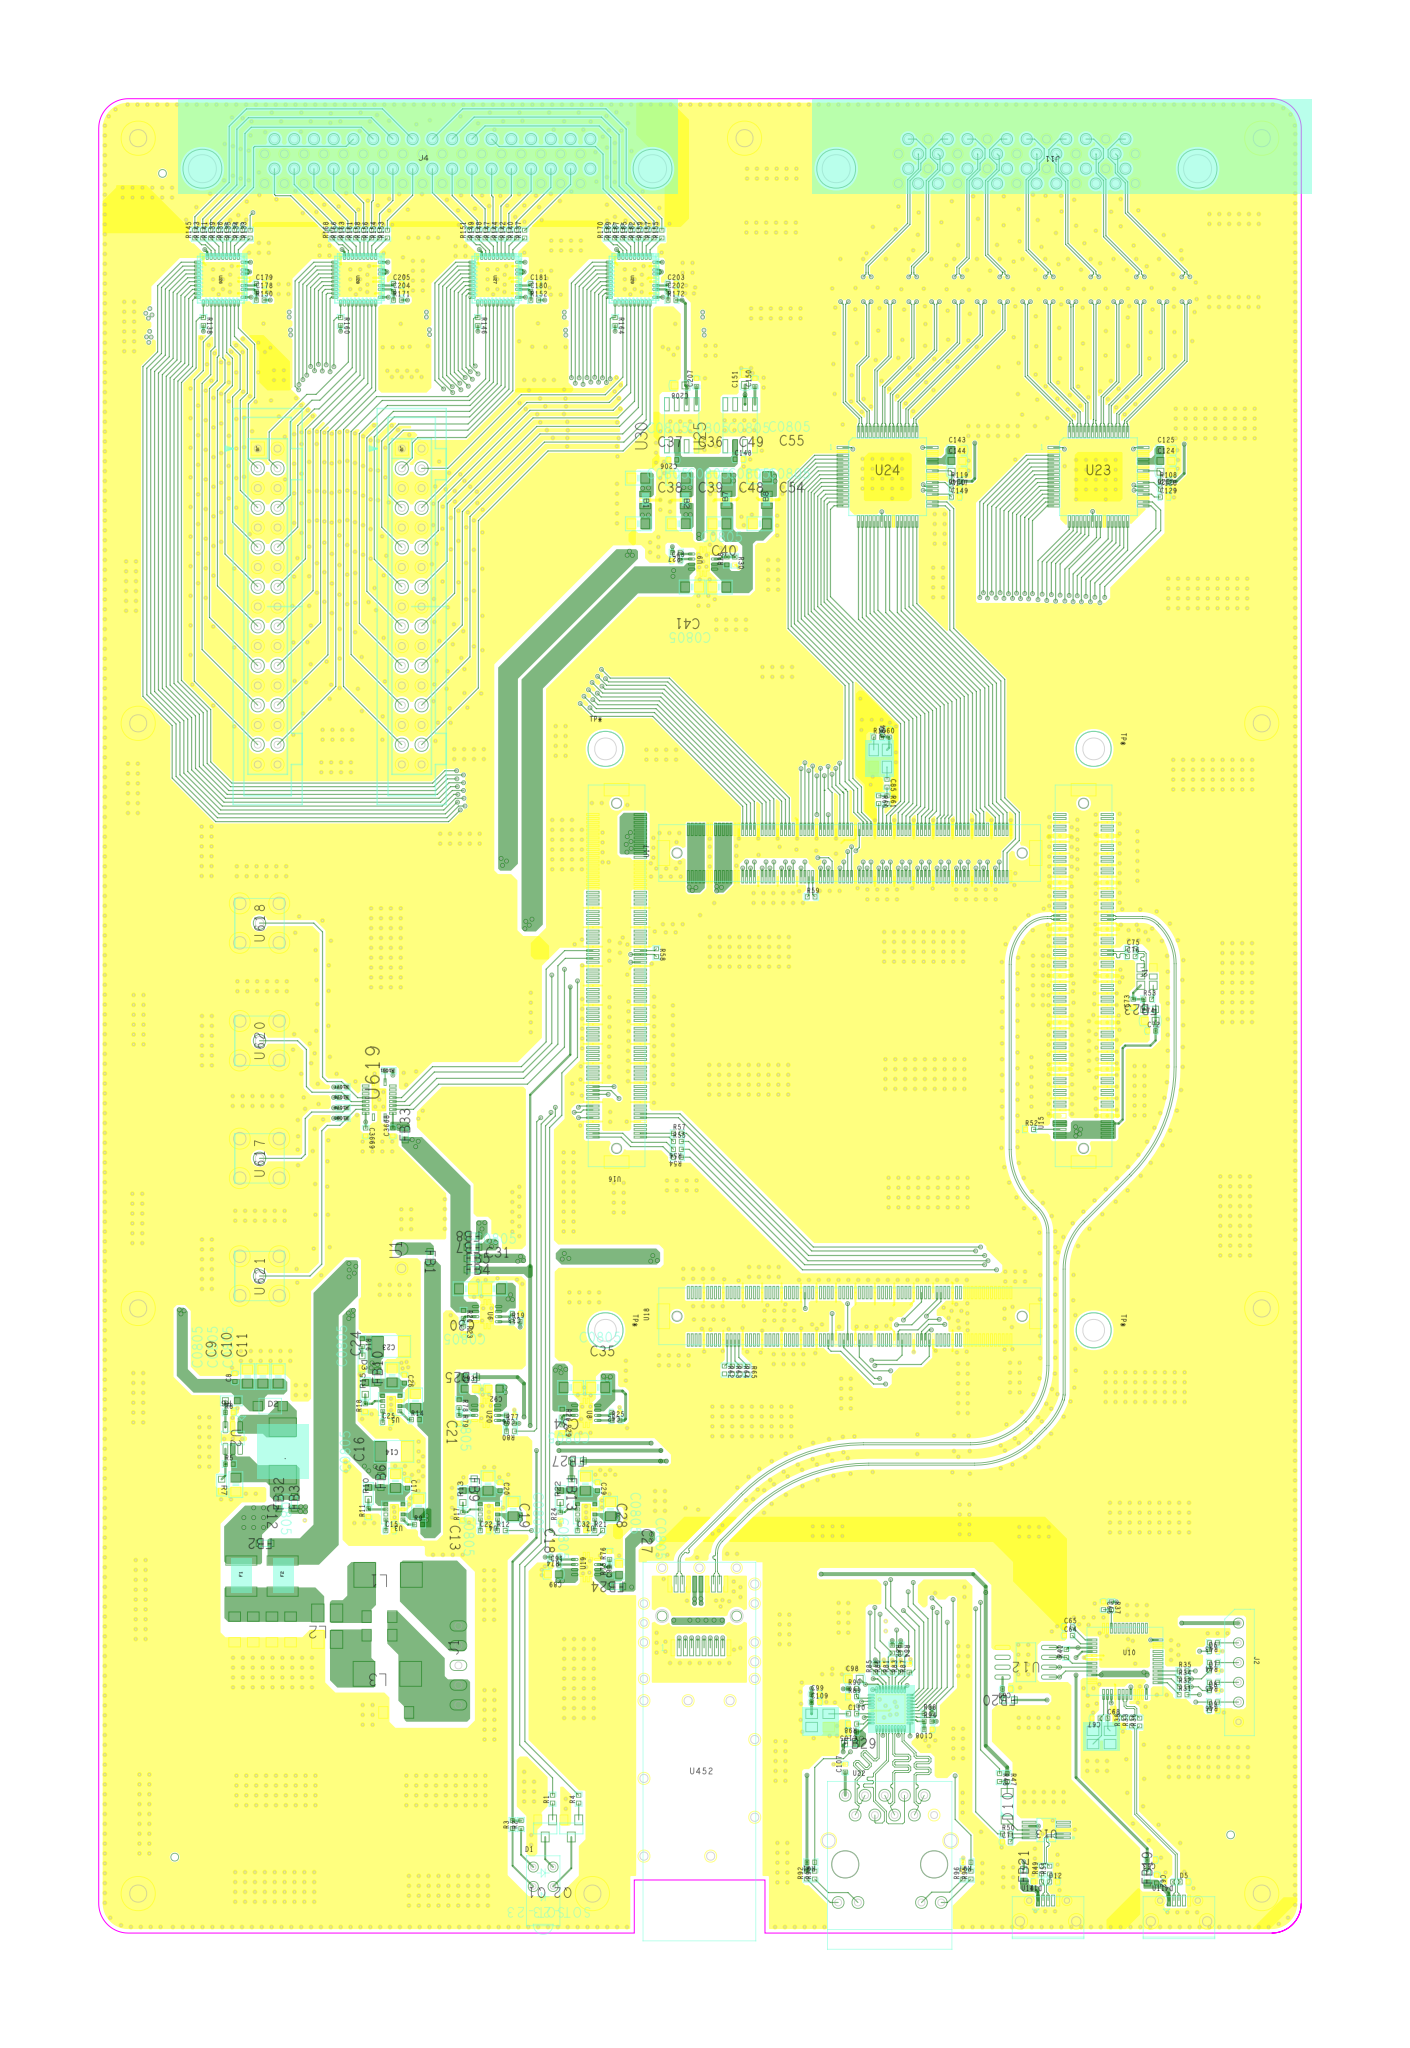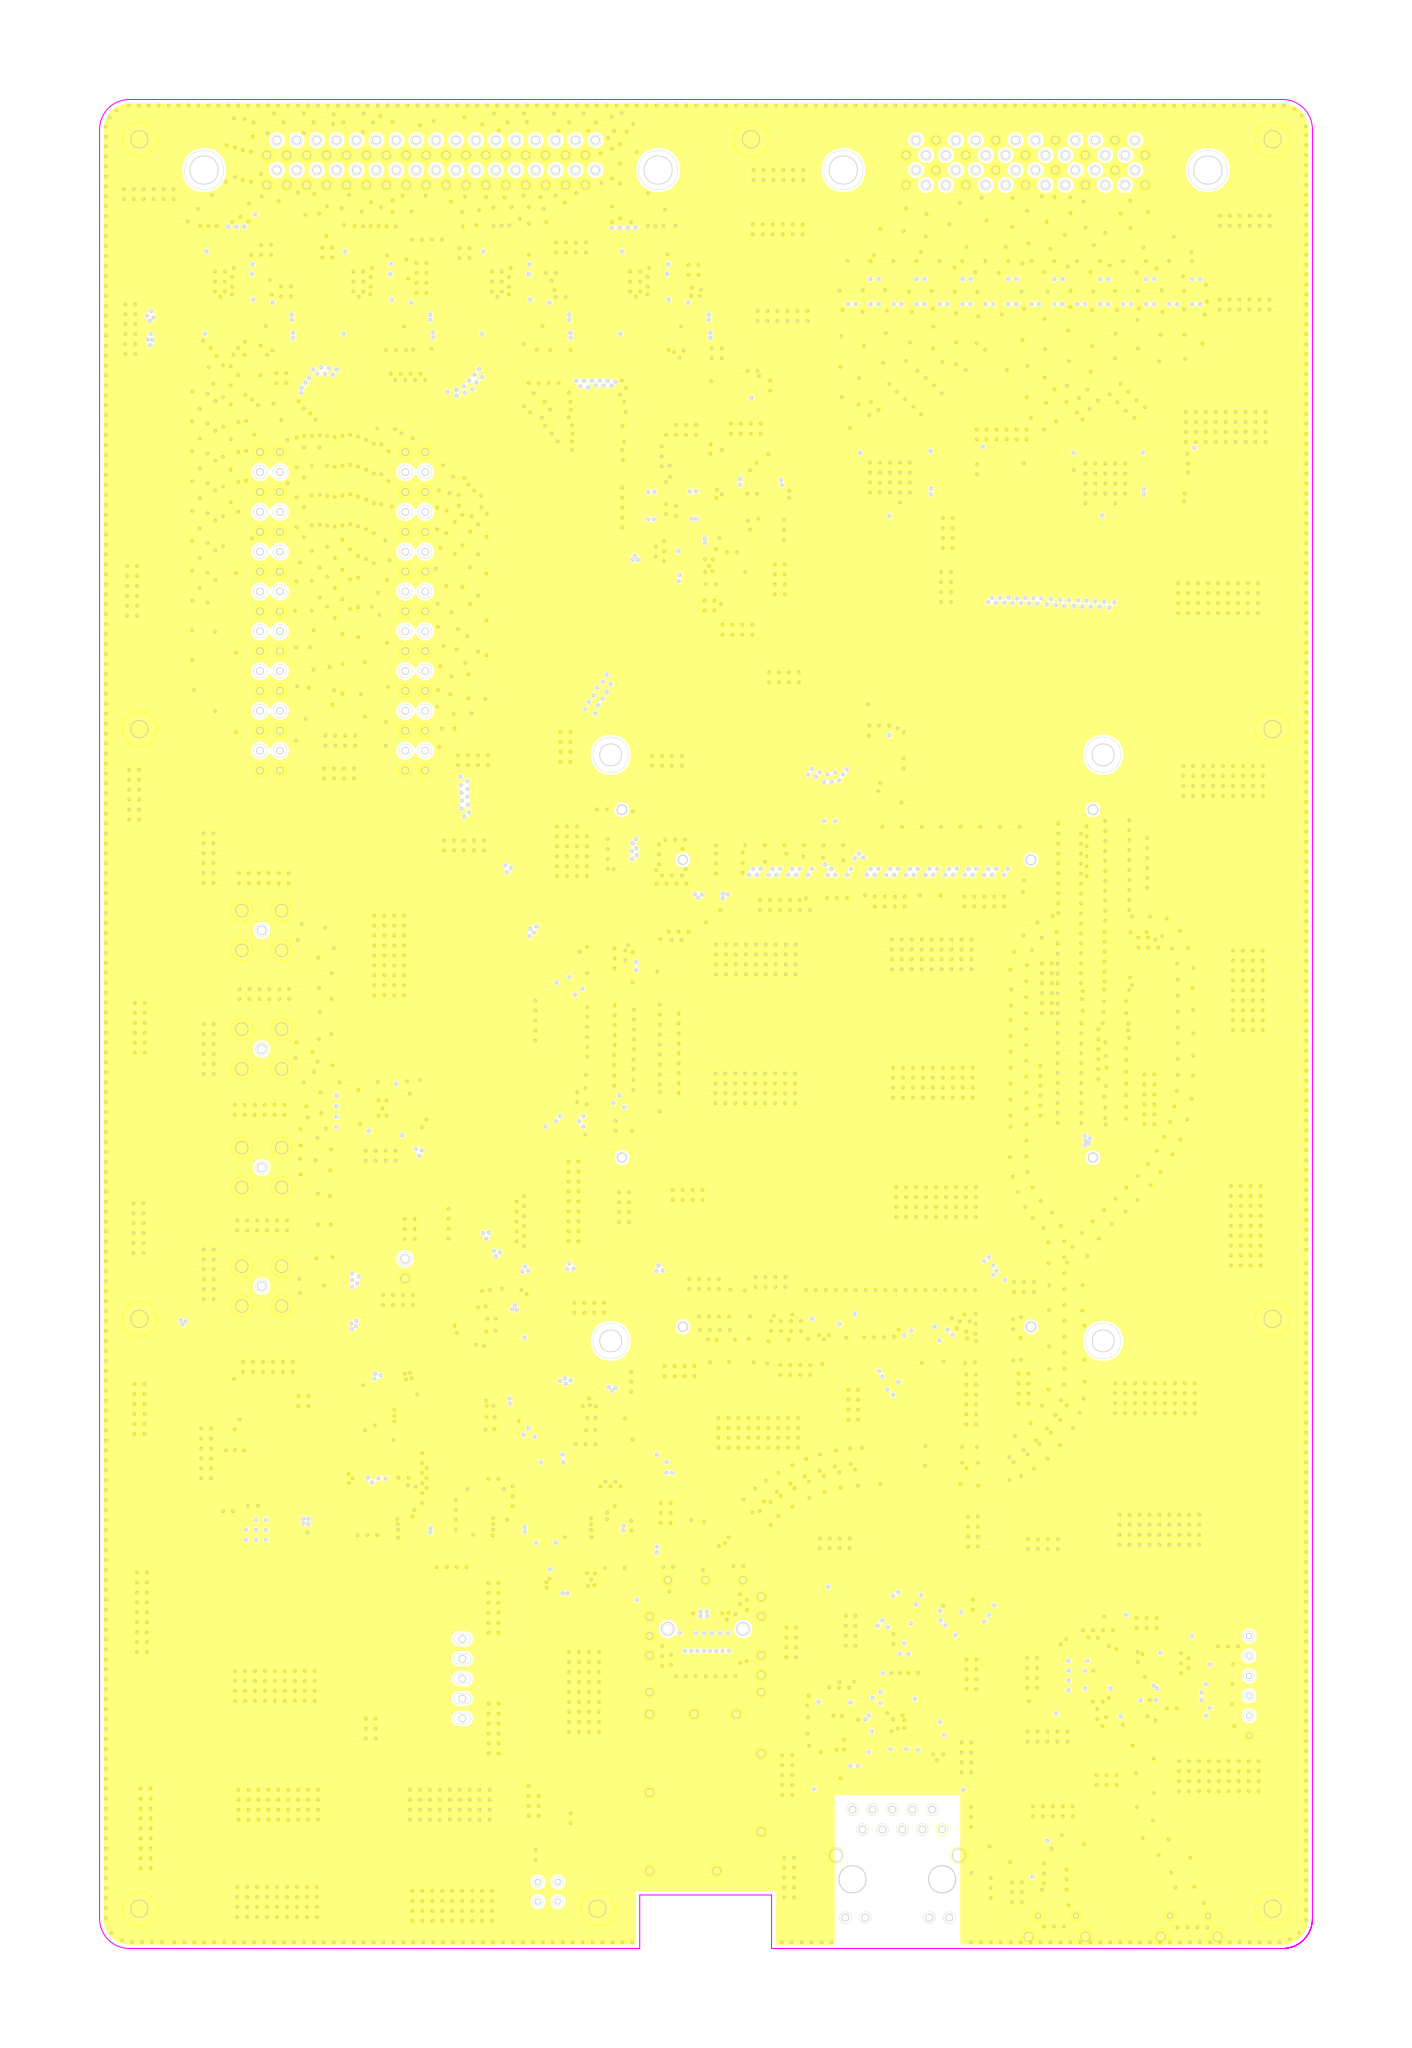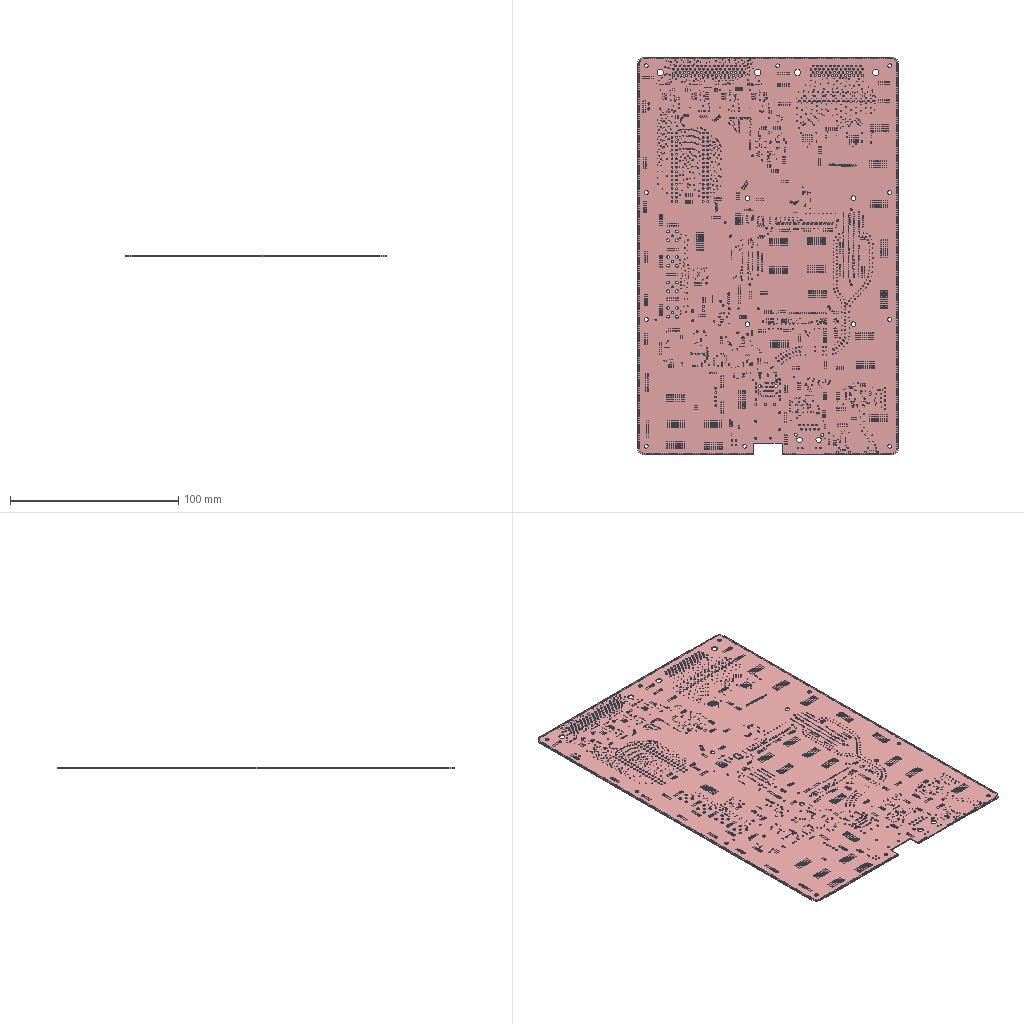Circuit board layout | Cadence Allegro | box 154.7 x 236 x 0.7 mm
Layer stack:
# Cadence Allegro layer stack of  (unit mm; from the constraint file cross-section; dielectric type: 0 not recorded (Allegro does not mark core vs prepreg), 3 surface material)
index,name,kind,layer,copper_thickness_mm,dielectric_type,dielectric_thickness_mm,dielectric_material,dielectric_constant
0,Top Surface,other,,,,,,
1,TOP,copper,TOP,0.0305,,,,
2,Dielectric1,dielectric,,,0,0.2032,FR-4,4.5
3,GND02,copper,GND02,0.0305,,,,
4,Dielectric2,dielectric,,,0,0.2032,FR-4,4.5
5,POWER03,copper,POWER03,0.0305,,,,
6,Dielectric3,dielectric,,,0,0.2032,FR-4,4.5
7,BOTTOM,copper,BOTTOM,0.0305,,,,
8,Bottom Surface,other,,,,,,
# drill layer pairs: low layer,high layer
drill_pair,TOP,BOTTOM
Part placement:
REFDES,COMP_VALUE,SYM_NAME,SYM_X,SYM_Y,SYM_ROTATE,SYM_MIRROR
B1,NFM18PS105R0J3D,B0603,-9307.660,8216.771,270.000,NO
B2,NFM18PS105R0J3D,B0603,-9102.919,8216.771,270.000,NO
B3,NFM18PS105R0J3D,B0603,-11211.472,9034.427,0.000,YES
B4,NFM18PS105R0J3D,B0603,-9821.236,9034.427,0.000,YES
B5,NFM18PS105R0J3D,B0603,-10516.353,9034.428,0.000,YES
B6,NFM18PS105R0J3D,B0603,-9126.118,9034.427,0.000,YES
B7,NFM18PS105R0J3D,B0603,-8896.604,8159.291,90.000,NO
B8,NFM18PS105R0J3D,B0603,-8691.863,8159.291,90.000,NO
B9,NFM18PS105R0J3D,B0603,-11211.472,9127.394,0.000,YES
B10,NFM18PS105R0J3D,B0603,-9821.236,9127.394,0.000,YES
B11,NFM18PS105R0J3D,B0603,-10516.353,9127.395,0.000,YES
B12,NFM18PS105R0J3D,B0603,-9126.118,9127.394,0.000,YES
C1,1000pF/1KV,C1206,-10653.465,2532.102,180.000,NO
C2,47uF/25V,C1206,-11386.967,2467.055,90.000,NO
C3,47uF/25V,C1206,-11292.588,2467.055,90.000,NO
C4,47uF/25V,C1206,-11198.209,2467.054,90.000,NO
C5,47uF/25V,C1206,-11103.830,2467.051,90.000,NO
C6,1000pF/1KV,C1206,-10653.465,2437.972,0.000,NO
C7,1000pF/1KV,C1206,-10568.831,2046.598,180.000,NO
C8,100nF,C0402,-11385.515,3742.780,90.000,NO
C9,22uF/25v,C0805,-11321.690,3747.951,90.000,NO
C10,22uF/25v,C0805,-11244.091,3747.951,90.000,NO
C11,22uF/25v,C0805,-11166.351,3747.951,90.000,NO
C12,22uF/25v,C0805,-11380.992,3200.522,270.000,NO
C13,10uF/25v,C0805,-10454.996,3093.283,270.000,NO
C14,100uF/10V,C1210,-10579.878,3368.803,180.000,NO
C15,3.3nF,C0402,-10601.579,2968.028,0.000,NO
C16,10uF/10v,C0805,-10572.587,3218.803,90.000,NO
C17,100nF,C0402,-10511.638,3203.122,270.000,NO
C18,10uF/25v,C0805,-9976.343,3076.067,270.000,NO
C19,10uF,C0805,-10103.472,3205.098,270.000,NO
C20,100nF,C0402,-10042.594,3189.787,270.000,NO
C21,10uF/25v,C0805,-10470.815,3624.908,270.000,NO
C22,3.3nF,C0402,-10122.925,2968.028,0.000,NO
C23,100uF/10V,C1210,-10595.696,3900.428,180.000,NO
C24,10uF,C0805,-10589.326,3753.538,90.000,NO
C25,3.3nF,C0402,-10617.397,3516.869,0.000,NO
C26,100nF,C0402,-10527.456,3734.751,270.000,NO
C27,10uF/25v,C0805,-9483.406,3076.067,270.000,NO
C28,10uF,C0805,-9610.535,3205.098,270.000,NO
C29,100nF,C0402,-9549.657,3189.787,270.000,NO
C30,10uF,C0805,-10073.378,4192.627,180.000,NO
C31,10uF,C0805,-10215.390,4192.627,0.000,NO
C32,3.3nF,C0402,-9629.988,2968.028,0.000,NO
C33,10nF,C0402,-9960.610,4065.904,180.000,NO
C34,10uF,C0805,-9545.416,3692.627,180.000,NO
C35,10uF,C0805,-9685.559,3692.627,0.000,NO
C36,47uF,C0805,-9137.919,8298.555,0.000,NO
C37,47uF,C0805,-9342.660,8298.555,0.000,NO
C38,22uF,C0805,-9342.660,8067.383,0.000,NO
C39,22uF,C0805,-9137.919,8067.383,0.000,NO
C40,10uF,C0805,-9070.145,7747.089,0.000,NO
C41,10uF,C0805,-8932.173,7746.453,180.000,NO
C42,10nF,C0402,-9457.319,3565.904,180.000,NO
C43,10nF,C0402,-9150.441,7880.702,0.000,NO
C44,22uF,C0805,-11370.868,9096.955,180.000,YES
C45,47uF,C0805,-9058.005,8999.427,270.000,YES
C46,22uF,C0805,-10675.749,9096.956,180.000,YES
C47,47uF,C0805,-11143.359,8999.427,270.000,YES
C48,47uF,C0805,-8931.604,8067.383,0.000,NO
C49,22uF,C0805,-8931.604,8298.555,0.000,NO
C50,47uF,C0805,-9753.123,8999.427,270.000,YES
C51,22uF,C0805,-9980.632,9096.955,180.000,YES
C52,47uF,C0805,-10448.240,8999.428,270.000,YES
C53,22uF,C0805,-9285.514,9096.955,180.000,YES
C54,47uF,C0805,-8726.863,8067.383,0.000,NO
C55,22uF,C0805,-8726.863,8305.031,0.000,NO
C56,100nF,C0402,-6975.679,2149.165,180.000,YES
C57,100nF,C0402,-6848.022,2219.803,90.000,YES
C58,100nF,C0402,-6788.970,2413.846,0.000,YES
C59,100nF,C0402,-6789.051,2206.611,0.000,YES
C60,100nF,C0402,-7042.840,2249.665,0.000,YES
C61,4.7uF,C0603,-6800.813,2364.484,0.000,YES
C62,100nF,C0402,-6717.352,1202.654,270.000,NO
C63,100nF,C0402,-6745.234,1299.941,180.000,NO
C64,100nF,C0402,-7164.124,2436.039,0.000,NO
C65,100nF,C0402,-7164.124,2479.327,0.000,NO
C66,100nF,C0402,-6986.703,2586.965,270.000,NO
C67,20pF,C0402,-7023.801,2017.671,180.000,NO
C68,20pF,C0402,-6944.880,2017.671,0.000,NO
C69,100nF,C0402,-7478.035,2165.541,180.000,NO
C70,100nF,C0402,-7274.913,1470.584,0.000,YES
C71,100nF,C0402,-7478.531,1391.480,0.000,NO
C72,100nF,C0402,-6742.232,5498.634,0.000,NO
C73,100nF,C0402,-6836.008,5639.425,90.000,NO
C74,4.7uF,C0603,-6750.023,5549.752,0.000,NO
C75,100nF,C0402,-6845.806,5915.077,0.000,NO
C76,100nF,C0402,-6845.806,5875.939,0.000,NO
C77,4.7uF/25V,C0603,-9461.460,6392.133,180.000,YES
C78,4.7uF/25V,C0603,-9461.460,6451.172,180.000,YES
C79,4.7uF/25V,C0603,-9461.460,6507.971,180.000,YES
C80,100nF,C0402,-9328.191,6386.937,0.000,YES
C81,100nF,C0402,-9328.191,6427.075,0.000,YES
C82,100nF,C0402,-9328.191,6467.209,0.000,YES
C83,100nF,C0402,-9328.191,6507.346,0.000,YES
C84,100nF,C0402,-8072.260,7006.806,90.000,NO
C85,100nF,C0402,-8083.014,6753.360,270.000,NO
C89,10uF,C0603,-9772.652,2746.604,180.000,NO
C90,10uF,C0603,-9439.415,2771.304,90.000,NO
C91,10nF,C0402,-9764.861,2793.770,0.000,NO
C92,10uF,C0603,-10073.435,3686.213,180.000,NO
C93,10uF,C0603,-10193.706,3686.213,0.000,NO
C94,4.7uF,C0603,-8206.554,2268.255,180.000,YES
C95,100nF,C0402,-8206.227,2219.187,0.000,YES
C96,10nF,C0402,-9990.212,3551.331,180.000,NO
C97,100nF,C0402,-8037.125,1986.260,270.000,YES
C98,4.7uF,C0603,-8248.514,2217.170,0.000,NO
C99,100nF,C0402,-8445.241,2138.735,0.000,NO
C100,100nF,C0402,-8137.952,2003.831,180.000,YES
C101,100nF,C0402,-8076.665,1986.260,270.000,YES
C102,4.7uF,C0603,-8124.873,2051.650,0.000,YES
C103,4.7uF,C0603,-8079.685,2136.647,270.000,YES
C104,100nF,C0402,-8029.536,2147.466,90.000,YES
C105,100nF,C0402,-8257.582,1948.509,180.000,NO
C106,100nF,C0402,-7913.783,1945.001,180.000,YES
C107,100nF,C0402,-8294.390,1764.417,90.000,NO
C108,100nF,C0402,-7874.984,1961.678,180.000,NO
C109,100nF,C0402,-8445.189,2098.814,0.000,NO
C110,100nF,C0402,-8257.582,2039.631,0.000,NO
C111,24nF,C0402,-6569.403,9217.760,180.000,YES
C112,100nF,C0402,-7164.657,8404.154,90.000,YES
C113,100nF,C0402,-7204.657,8404.154,90.000,YES
C114,100nF,C0402,-6880.501,8395.984,0.000,YES
C115,10nF,C0402,-6880.501,8355.984,0.000,YES
C116,100pF,C0402,-6880.501,8279.984,0.000,YES
C117,10pF,C0402,-6880.501,8240.555,0.000,YES
C118,47uF,C0603,-6884.202,8191.992,0.000,YES
C119,100nF,C0402,-7063.165,8171.238,270.000,YES
C120,100nF,C0402,-7021.496,8171.238,270.000,YES
C121,24nF,C0402,-6684.675,9217.760,180.000,YES
C122,24nF,C0402,-6799.947,9217.760,180.000,YES
C123,24nF,C0402,-6915.219,9217.760,180.000,YES
C124,22uF,C0603,-6670.588,8385.670,0.000,NO
C125,22uF,C0603,-6670.588,8440.693,0.000,NO
C126,10uF,C0603,-6670.588,8330.930,180.000,NO
C127,24nF,C0402,-7030.491,9217.760,180.000,YES
C128,1uF,C0402,-6678.379,8242.961,0.000,NO
C129,1uF,C0402,-6678.379,8203.060,0.000,NO
C130,24nF,C0402,-7145.763,9217.760,180.000,YES
C131,24nF,C0402,-7261.035,9217.760,180.000,YES
C132,100nF,C0402,-8234.109,8404.010,90.000,YES
C133,100nF,C0402,-8274.109,8404.010,90.000,YES
C134,100nF,C0402,-7959.997,8408.200,0.000,YES
C135,10nF,C0402,-7959.997,8368.200,0.000,YES
C136,100pF,C0402,-7964.725,8298.104,0.000,YES
C137,10pF,C0402,-7964.725,8258.675,0.000,YES
C138,47uF,C0603,-7968.426,8210.112,0.000,YES
C139,100nF,C0402,-8129.509,8171.094,270.000,YES
C140,100nF,C0402,-8087.840,8171.094,270.000,YES
C141,24nF,C0402,-7376.307,9217.760,180.000,YES
C142,24nF,C0402,-7491.579,9217.760,180.000,YES
C143,22uF,C0603,-7728.416,8440.693,0.000,NO
C144,22uF,C0603,-7728.416,8385.670,0.000,NO
C145,24nF,C0402,-7606.851,9217.760,180.000,YES
C146,10uF,C0603,-7728.416,8330.930,180.000,NO
C147,1uF,C0402,-7736.207,8242.961,0.000,NO
C148,1uF,C0402,-8832.647,8394.406,0.000,NO
C149,1uF,C0402,-7736.207,8203.060,0.000,NO
C150,1uF,C0402,-8751.992,8782.930,90.000,NO
C151,22uF,C0603,-8801.901,8798.300,90.000,NO
C152,24nF,C0402,-7722.123,9217.760,180.000,YES
C153,24nF,C0402,-7837.395,9217.760,180.000,YES
C154,24nF,C0402,-7952.667,9217.760,180.000,YES
C155,24nF,C0402,-8183.211,9217.760,180.000,YES
C156,24nF,C0402,-8067.939,9217.760,180.000,YES
C157,24nF,C0402,-8298.483,9217.760,180.000,YES
C158,47uF,C0603,-11143.947,9164.690,90.000,YES
C159,22uF,C0603,-11247.308,9274.775,0.000,YES
C160,47uF,C0603,-9753.711,9164.690,90.000,YES
C161,22uF,C0603,-9857.072,9274.775,0.000,YES
C162,100nF,C0402,-11359.535,9329.894,0.000,YES
C163,10nF,C0402,-11359.535,9290.197,0.000,YES
C164,100pF,C0402,-11359.535,9250.555,0.000,YES
C165,47uF,C0603,-11379.335,9202.905,0.000,YES
C166,100nF,C0402,-11257.484,9200.445,180.000,YES
C167,100nF,C0402,-11257.484,9376.993,180.000,YES
C168,100nF,C0402,-11518.550,9388.673,180.000,YES
C169,100nF,C0402,-11518.550,9427.291,180.000,YES
C170,100nF,C0402,-9969.299,9329.894,0.000,YES
C171,10nF,C0402,-9969.299,9290.197,0.000,YES
C172,100pF,C0402,-9969.299,9250.555,0.000,YES
C173,47uF,C0603,-9989.099,9202.905,0.000,YES
C174,100nF,C0402,-9867.248,9376.993,180.000,YES
C175,100nF,C0402,-9867.248,9200.445,180.000,YES
C176,100nF,C0402,-10128.314,9388.673,180.000,YES
C177,100nF,C0402,-10128.314,9427.291,180.000,YES
C178,150nF,C0402,-11257.484,9242.295,0.000,NO
C179,330pF,C0402,-11257.484,9283.770,0.000,NO
C180,150nF,C0402,-9867.248,9242.295,0.000,NO
C181,330pF,C0402,-9867.248,9283.770,0.000,NO
C182,47uF,C0603,-10448.828,9164.691,90.000,YES
C183,22uF,C0603,-10552.189,9274.776,0.000,YES
C184,47uF,C0603,-9058.593,9164.690,90.000,YES
C185,22uF,C0603,-9161.954,9274.775,0.000,YES
C186,100nF,C0402,-10664.416,9329.895,0.000,YES
C187,10nF,C0402,-10664.416,9290.198,0.000,YES
C188,100pF,C0402,-10664.416,9250.556,0.000,YES
C189,47uF,C0603,-10684.216,9202.906,0.000,YES
C190,100nF,C0402,-10562.365,9376.994,180.000,YES
C191,100nF,C0402,-10562.365,9200.446,180.000,YES
C192,100nF,C0402,-10823.431,9427.292,180.000,YES
C193,100nF,C0402,-10823.431,9388.674,180.000,YES
C194,100nF,C0402,-9274.181,9329.894,0.000,YES
C195,10nF,C0402,-9274.181,9290.197,0.000,YES
C196,100pF,C0402,-9274.181,9250.555,0.000,YES
C197,47uF,C0603,-9293.981,9202.905,0.000,YES
C198,100nF,C0402,-9172.130,9376.993,180.000,YES
C199,100nF,C0402,-9172.130,9200.445,180.000,YES
C200,100nF,C0402,-9433.196,9427.291,180.000,YES
C201,100nF,C0402,-9433.196,9388.673,180.000,YES
C202,150nF,C0402,-9172.130,9242.295,0.000,NO
C203,330pF,C0402,-9172.130,9283.770,0.000,NO
C204,150nF,C0402,-10562.365,9242.296,0.000,NO
C205,330pF,C0402,-10562.365,9283.771,0.000,NO
C206,1uF,C0402,-9167.871,8391.351,180.000,NO
C207,1uF,C0402,-9047.884,8782.930,90.000,NO
C208,22uF,C0603,-9131.416,8768.208,180.000,NO
C3194,22uF,C0603,-9075.849,3014.611,270.000,YES
C3197,22uF,C0603,-9088.165,2655.335,0.000,YES
C3202,0.1uF,C0402,-8969.042,2707.217,0.000,YES
C3203,22uF,C0603,-8970.323,2655.335,180.000,YES
C3666,0.1uF,C0402,-9010.711,3009.934,90.000,YES
C3667,0.1uF,C0402,-9086.566,2707.217,180.000,YES
C3668,100nF,C0402,-10585.688,4986.800,90.000,NO
C3669,100nF,C0402,-10723.409,4986.800,270.000,NO
D1,MHK2396YGYGBTD,MHK2396YGYGBTD,-9874.339,1263.543,0.000,NO
D2,DSK24,DSK24,-11206.792,3598.279,0.000,NO
D3,LN211WP,D0603,-10741.369,3821.677,270.000,NO
D4,BPESD0402,C0402,-6656.274,1188.183,180.000,NO
D5,BPESD0402,C0402,-6578.006,1188.183,0.000,NO
D6,BPESD0402,C0402,-6429.561,2356.882,0.000,NO
D7,BPESD0402,C0402,-6429.561,2257.902,0.000,NO
D8,BPESD0402,C0402,-6429.561,2157.661,0.000,NO
D9,BPESD0402,C0402,-6429.561,2057.193,0.000,NO
D10,LL4148,SOD-80,-7474.070,1571.454,90.000,NO
D11,BPESD0402,C0402,-7320.263,1188.183,180.000,NO
D12,BPESD0402,C0402,-7239.464,1188.183,0.000,NO
F1,NC/BSMD1812P300TF/16V,SMD1812,-11353.224,2658.512,90.000,NO
F2,BSMD1812P300TF/16V,SMD1812,-11143.933,2658.512,90.000,NO
FB1,BLM18PG121SN1,0603,-10397.390,4351.832,270.000,NO
FB2,BLM18PG121SN1,0603,-11232.969,2903.211,180.000,NO
FB3,BLM18PG121SN1,0603,-11084.048,3110.585,90.000,NO
FB4,BLM18PG121SN1,0603,-10180.087,4288.957,0.000,NO
FB5,NC,0603,-10180.087,4345.898,0.000,NO
FB6,BLM18PG121SN1,0603,-10646.307,3216.004,90.000,NO
FB7,BLM18PG121SN1,0603,-10180.087,4402.839,180.000,NO
FB8,BLM18PG121SN1,0603,-10180.087,4459.780,180.000,NO
FB9,BLM18PG121SN1,0603,-10173.815,3200.020,270.000,NO
FB10,BLM18PG121SN1,0603,-10662.126,3747.629,90.000,NO
FB11,BLM18PG121SN1,0603,-9343.144,8803.405,90.000,YES
FB12,BLM18PG121SN1,0603,-9229.262,8803.405,90.000,YES
FB13,BLM18PG121SN1,0603,-9680.878,3200.020,270.000,NO
FB14,BLM18PG121SN1,0603,-9286.203,8803.405,90.000,YES
FB15,BLM18PG121SN1,0603,-9172.321,8803.405,90.000,YES
FB16,BLM18PG121SN1,0603,-6955.399,2230.307,90.000,YES
FB17,BLM18PG121SN1,0603,-6897.600,2230.035,90.000,YES
FB18,BLM18PG121SN1,0603,-6982.795,2318.585,0.000,YES
FB19,BLM18PG121SN1,0603,-6764.923,1212.886,90.000,NO
FB20,BLM18PG121SN1,0603,-7467.803,2109.680,180.000,NO
FB21,BLM18PG121SN1,0603,-7390.247,1222.389,90.000,NO
FB23,BLM18PG121SN1,0603,-6752.464,5607.996,180.000,NO
FB24,BLM18PG121SN1,0603,-9451.453,2684.391,180.000,NO
FB25,BLM18PG121SN1,0603,-10191.265,3744.975,180.000,NO
FB26,BLM18PG121SN1,0603,-7982.944,1997.871,90.000,YES
FB27,BLM18PG121SN1,0603,-9650.957,3320.653,180.000,NO
FB28,BLM18PG121SN1,0603,-7982.944,2117.268,90.000,YES
FB29,BLM18PG121SN1,0603,-8267.814,1888.976,0.000,NO
FB30,BLM18PG121SN1,FB0603,-9075.849,2888.450,90.000,YES
FB31,BLM18PG121SN1,FB0603,-9010.711,2888.450,90.000,YES
FB32,NC,0603,-11162.990,3108.133,90.000,NO
FB33,BLM18PG121SN1,0603,-10523.405,4976.568,90.000,NO
G1,NC/SiT9121-156.25MHz,OSC6-3225,-6765.964,5774.115,90.000,NO
H9,HOLE220D450,GMPTH2_2R4_4,-6184.909,1129.172,0.000,NO
H10,HOLE220D450,GMPTH2_2R4_4,-11875.460,1129.172,0.000,NO
H11,HOLE220D450,GMPTH2_2R4_4,-11875.459,7056.656,0.000,NO
H12,HOLE220D450,GMPTH2_2R4_4,-6184.909,7056.656,0.000,NO
H13,HOLE220D450,GMPTH2_2R4_4,-6184.909,10020.398,0.000,NO
H14,HOLE220D450,GMPTH2_2R4_4,-6184.909,4092.914,0.000,NO
H15,HOLE220D450,GMPTH2_2R4_4,-11875.459,10020.398,0.000,NO
H16,HOLE220D450,GMPTH2_2R4_4,-11875.459,4092.914,0.000,NO
H17,HOLE220D450,GMPTH2_2R4_4,-9575.098,1129.172,0.000,NO
H18,HOLE220D450,GMPTH2_2R4_4,-8804.584,10020.398,0.000,NO
J1,HDR5,2R54_5P,-10253.724,2335.024,270.000,NO
J2,HDR6,HDR6-254MM,-6302.683,2499.201,270.000,NO
J4,CONN SCSI68,SCSI68,-11367.051,9960.193,0.000,NO
J8,HEADER 17X2,CONN-TH_XH2_5-34P,-11269.888,8448.186,270.000,NO
J9,HEADER 17X2,CONN-TH_XH2_5-34P,-10540.286,8448.186,270.000,NO
J11,CONN CENT 50,SCSI50,-5872.980,10054.083,180.000,NO
L1,FXL0630_1R5_M,SMD_SMD_7X6_6,-10609.815,2743.484,180.000,NO
L2,SRF0504-191Y,SFC-BNX027,-10918.350,2483.476,180.000,NO
L3,FXL0630_1R5_M,SMD_SMD_7X6_6,-10613.547,2242.063,180.000,NO
L4,MWSA0603S-8R2MT,PL0603,-11143.142,3371.183,90.000,NO
OSC-25M2,25MHz,3225-4,-8421.452,2006.170,0.000,NO
Q1,BSN20,SOT-23,-9814.091,1459.142,180.000,NO
Q2,BSN20,SOT-23,-9681.890,1459.142,180.000,NO
R1,33R,R0402,-9776.689,1607.370,90.000,NO
R2,510R,R0402,-9936.362,1478.862,90.000,NO
R3,510R,R0402,-9979.374,1478.862,90.000,NO
R4,33R,R0402,-9644.488,1607.370,90.000,NO
R5,10k,R0402,-11414.102,3304.242,0.000,NO
R6,240K,R0603,-11403.831,3624.931,180.000,NO
R7,1M,R0603,-11452.823,3197.842,270.000,NO
R8,10k,R0402,-11414.142,3566.281,0.000,NO
R9,1k,R0402,-10455.768,2998.374,0.000,NO
R10,590k,R0603,-10709.748,3156.083,90.000,NO
R11,100k,R0402,-10709.748,3058.594,90.000,NO
R12,100R,R0402,-10036.303,2968.028,0.000,NO
R13,215k,R0603,-10231.094,3140.098,90.000,NO
R14,1k,R0402,-10471.586,3529.999,0.000,NO
R15,383k,R0603,-10725.555,3687.940,90.000,NO
R16,2.49K/1%,R0402,-10741.369,3919.559,270.000,NO
R17,100k,R0402,-10231.094,3041.378,90.000,NO
R18,100k,R0402,-10725.566,3590.219,90.000,NO
R19,10k,R0402,-9960.610,4025.740,0.000,NO
R20,30.9k,R0402,-10228.098,4062.579,270.000,NO
R21,100R,R0402,-9543.366,2968.028,0.000,NO
R22,127k,R0603,-9738.157,3140.098,90.000,NO
R23,10k,R0402,-10228.098,3983.650,270.000,NO
R24,100k,R0402,-9738.157,3041.378,90.000,NO
R25,10k,R0402,-9455.035,3525.740,0.000,NO
R26,52.3k,R0402,-9728.236,3562.579,270.000,NO
R27,10k,R0402,-9150.441,7921.616,180.000,NO
R28,52.3k,R0402,-8893.780,7879.403,90.000,NO
R29,10k,R0402,-9728.236,3483.650,270.000,NO
R30,10k,R0402,-8853.642,7878.899,270.000,NO
R31,33R,R0402,-6583.490,2136.685,0.000,NO
R32,33R,R0402,-6583.490,2176.685,0.000,NO
R33,33R,R0402,-6843.548,1998.038,90.000,NO
R34,33R,R0402,-6583.490,2216.685,0.000,NO
R35,33R,R0402,-6583.490,2256.685,0.000,NO
R36,33R,R0402,-6803.458,1998.038,90.000,NO
R37,10k,R0402,-6946.762,2586.965,270.000,NO
R38,10k,R0402,-6884.627,1998.038,90.000,NO
R39,10k,R0402,-7255.060,2225.840,0.000,YES
R40,10k,R0402,-7255.060,2275.840,0.000,YES
R41,10k,R0402,-7174.879,2345.529,90.000,NO
R42,2k,R0402,-7235.371,2345.529,270.000,YES
R43,33R,R0402,-6429.561,2399.201,180.000,NO
R44,33R,R0402,-6429.561,2299.201,180.000,NO
R45,33R,R0402,-6429.561,2199.201,180.000,NO
R46,33R,R0402,-6429.561,2099.201,180.000,NO
R47,100k,R0402,-7474.070,1716.817,270.000,NO
R48,1k,R0402,-7512.869,1716.817,270.000,NO
R49,33R,R0402,-7300.574,1248.353,90.000,NO
R50,1k,R0402,-7478.531,1431.474,0.000,NO
R51,33R,R0402,-7259.153,1248.353,90.000,NO
R52,0R,R0402,-7360.909,5000.075,0.000,NO
R53,4.7k,R0402,-6762.697,5659.114,0.000,NO
R54,33R,R0402,-9144.618,4859.058,180.000,NO
R55,33R,R0402,-9144.618,4938.828,0.000,NO
R56,33R,R0402,-9144.618,4899.109,180.000,NO
R57,33R,R0402,-9144.618,4980.088,0.000,NO
R58,DNI,R0402,-9251.307,5894.657,270.000,NO
R59,0R,R0402,-8467.135,6177.555,0.000,NO
R60,0R,R0402,-8125.305,6669.801,270.000,NO
R61,DNI,R0402,-8083.014,6669.801,270.000,NO
R62,DNI/33R,R0402,-8906.020,3781.315,270.000,NO
R63,DNI/33R,R0402,-8866.701,3781.315,270.000,NO
R64,DNI/33R,R0402,-8827.661,3781.315,270.000,NO
R65,DNI/33R,R0402,-8788.280,3780.094,270.000,NO
R74,10k,R0402,-9764.861,2833.474,180.000,NO
R75,30.9k,R0402,-9488.348,2763.513,90.000,NO
R76,10k,R0402,-9488.348,2841.647,90.000,NO
R77,10k,R0402,-9990.212,3510.556,0.000,NO
R78,30.9k,R0402,-10250.499,3610.492,270.000,NO
R79,10k,R0402,-10250.499,3531.642,270.000,NO
R80,NC,R0402,-9990.212,3471.450,180.000,NO
R81,47k/NC,R0402,-8056.484,2270.398,90.000,NO
R82,47k/NC,R0402,-8056.484,2367.172,270.000,NO
R83,47k/NC,R0402,-8013.637,2270.398,90.000,NO
R84,47k/NC,R0402,-8013.637,2367.172,270.000,NO
R85,10K,R0402,-8142.173,2270.398,90.000,NO
R86,10K,R0402,-8099.330,2270.398,90.000,NO
R87,10K,R0402,-7970.795,2270.398,90.000,NO
R88,10K,R0402,-7875.495,2042.119,0.000,NO
R89,NC/4.7k,R0402,-8257.353,2126.761,0.000,NO
R90,4.7k,R0402,-8257.353,2167.631,0.000,NO
R91,4.7k,R0402,-8468.780,1288.094,180.000,NO
R92,510R,R0402,-8489.402,1222.610,90.000,NO
R93,0R,R0402,-8449.091,1222.610,90.000,NO
R94,4.7k,R0402,-7874.984,2001.351,0.000,NO
R95,0R,R0402,-7657.768,1222.610,90.000,NO
R96,510R,R0402,-7698.535,1222.610,90.000,NO
R97,4.7k,R0402,-7677.457,1288.094,180.000,NO
R98,2.49K/1%,R0402,-8257.582,1988.028,180.000,NO
R99,10K,R0402,-6548.992,9276.480,270.000,YES
R100,10K,R0402,-6589.982,9276.078,270.000,YES
R101,10K,R0402,-6664.264,9276.480,270.000,YES
R102,10K,R0402,-6705.254,9276.078,270.000,YES
R103,10K,R0402,-6779.536,9276.480,270.000,YES
R104,10K,R0402,-6820.526,9276.078,270.000,YES
R105,10K,R0402,-6894.808,9276.480,270.000,YES
R106,10K,R0402,-6935.798,9276.078,270.000,YES
R107,10K,R0402,-7010.080,9276.480,270.000,YES
R108,NC,R0402,-6678.379,8282.733,0.000,NO
R109,10K,R0402,-7051.070,9276.078,270.000,YES
R110,10K,R0402,-7125.352,9276.480,270.000,YES
R111,10K,R0402,-7166.342,9276.078,270.000,YES
R112,10K,R0402,-7240.624,9276.480,270.000,YES
R113,10K,R0402,-7281.614,9276.078,270.000,YES
R114,10K,R0402,-7355.896,9276.480,270.000,YES
R115,10K,R0402,-7396.886,9276.078,270.000,YES
R116,10K,R0402,-7471.168,9276.480,270.000,YES
R117,10K,R0402,-7512.158,9276.078,270.000,YES
R118,10K,R0402,-7586.440,9276.480,270.000,YES
R119,NC,R0402,-7736.207,8282.733,0.000,NO
R120,10K,R0402,-7627.430,9276.078,270.000,YES
R121,10K,R0402,-7701.712,9276.480,270.000,YES
R122,10K,R0402,-7742.702,9276.078,270.000,YES
R123,10K,R0402,-7816.984,9276.480,270.000,YES
R124,10K,R0402,-7857.974,9276.078,270.000,YES
R125,10K,R0402,-7932.256,9276.480,270.000,YES
R126,10K,R0402,-8162.800,9276.480,270.000,YES
R127,10K,R0402,-7973.246,9276.078,270.000,YES
R128,10K,R0402,-8203.790,9276.078,270.000,YES
R129,10K,R0402,-8047.528,9276.480,270.000,YES
R130,10K,R0402,-8278.072,9276.480,270.000,YES
R131,10K,R0402,-8088.518,9276.078,270.000,YES
R132,10K,R0402,-8319.062,9276.078,270.000,YES
R133,0,R0402,-11308.622,9534.551,90.000,NO
R134,0,R0402,-11348.622,9534.551,90.000,NO
R135,0,R0402,-11388.622,9534.551,90.000,NO
R136,0,R0402,-11428.622,9534.551,90.000,NO
R137,0,R0402,-9918.386,9534.551,90.000,NO
R138,10K,R0402,-11545.436,9091.874,270.000,NO
R139,0,R0402,-11468.622,9534.551,90.000,NO
R140,0,R0402,-9958.386,9534.551,90.000,NO
R141,0,R0402,-11508.622,9534.551,90.000,NO
R142,0,R0402,-9998.386,9534.551,90.000,NO
R143,0,R0402,-11548.622,9534.551,90.000,NO
R144,0,R0402,-10038.386,9534.551,90.000,NO
R145,0,R0402,-11588.622,9534.551,90.000,NO
R146,10K,R0402,-10155.200,9091.874,270.000,NO
R147,0,R0402,-10078.386,9534.551,90.000,NO
R148,0,R0402,-10118.386,9534.551,90.000,NO
R149,0,R0402,-10158.386,9534.551,90.000,NO
R150,NC,R0402,-11257.484,9200.434,0.000,NO
R151,0,R0402,-10198.386,9534.551,90.000,NO
R152,NC,R0402,-9867.248,9200.434,0.000,NO
R153,0,R0402,-10613.503,9534.552,90.000,NO
R154,0,R0402,-10653.503,9534.552,90.000,NO
R155,0,R0402,-9223.268,9534.551,90.000,NO
R156,0,R0402,-10693.503,9534.552,90.000,NO
R157,0,R0402,-9263.268,9534.551,90.000,NO
R158,0,R0402,-10733.503,9534.552,90.000,NO
R159,0,R0402,-9303.268,9534.551,90.000,NO
R160,10K,R0402,-10850.317,9091.875,270.000,NO
R161,0,R0402,-10773.503,9534.552,90.000,NO
R162,0,R0402,-9343.268,9534.551,90.000,NO
R163,0,R0402,-10813.503,9534.552,90.000,NO
R164,10K,R0402,-9460.082,9091.874,270.000,NO
R165,0,R0402,-9383.268,9534.551,90.000,NO
R166,0,R0402,-10853.503,9534.552,90.000,NO
R167,0,R0402,-9423.268,9534.551,90.000,NO
R168,0,R0402,-10893.503,9534.552,90.000,NO
R169,0,R0402,-9463.268,9534.551,90.000,NO
R170,0,R0402,-9503.268,9534.551,90.000,NO
R171,NC,R0402,-10562.365,9200.435,0.000,NO
R172,NC,R0402,-9172.130,9200.434,0.000,NO
R240,4.7K,R0402,-8999.787,2469.744,270.000,YES
R241,4.7K,R0402,-9040.583,2469.744,270.000,YES
R242,4.7K,R0402,-9081.378,2469.744,270.000,YES
R243,4.7K,R0402,-9122.173,2469.744,270.000,YES
R244,4.7K,R0402,-9162.969,2469.744,270.000,YES
R246,4.7K,R0402,-8918.193,2469.744,270.000,YES
R247,4.7K,R0402,-8958.992,2469.744,270.000,YES
R1058,0R,R0402,-8858.744,2410.012,180.000,YES
R1059,NC,R0402,-8858.744,2449.173,180.000,YES
R1060,0R,R0402,-8130.472,6987.117,0.000,NO
R1061,0R,R0402,-6589.982,9361.060,270.000,YES
R1062,0R,R0402,-6705.254,9361.060,270.000,YES
R1063,0R,R0402,-6820.526,9361.060,270.000,YES
R1064,0R,R0402,-6935.798,9361.060,270.000,YES
R1065,0R,R0402,-7051.070,9361.060,270.000,YES
R1066,0R,R0402,-7166.342,9361.060,270.000,YES
R1067,0R,R0402,-7281.614,9361.060,270.000,YES
R1068,0R,R0402,-7396.886,9361.060,270.000,YES
R1069,0R,R0402,-7512.158,9361.060,270.000,YES
R1070,0R,R0402,-7627.430,9361.060,270.000,YES
R1071,0R,R0402,-7742.702,9361.060,270.000,YES
R1072,0R,R0402,-7857.974,9361.060,270.000,YES
R1073,0R,R0402,-7973.246,9361.060,270.000,YES
R1074,0R,R0402,-8088.518,9361.060,270.000,YES
R1075,0R,R0402,-8203.790,9361.060,270.000,YES
R1076,0R,R0402,-8319.062,9361.060,270.000,YES
R1077,4.7K,0402,-10837.672,5214.355,180.000,NO
R1078,4.7K,0402,-10837.672,5161.714,180.000,NO
R1079,4.7K,0402,-10837.672,5109.073,180.000,NO
R1080,4.7K,0402,-10837.672,5056.432,180.000,NO
R1081,4.7K,0402,-10605.295,5297.164,180.000,NO
U1,HDGC2501WV-2P,CONN-TH_XH2_5-2P,-10541.701,4345.240,90.000,NO
U2,SY7208LABC,SOT23-6,-11396.390,3436.612,270.000,NO
U3,TPS82130,SIL0008C,-10577.957,3062.118,180.000,NO
U4,TPS82130,SIL0008C,-10099.303,3062.118,180.000,NO
U5,TPS82130,SIL0008C,-10593.775,3610.959,180.000,NO
U6,TPS7A8001,TPS7A8001,-10108.528,4064.126,270.000,NO
U7,TPS82130,SIL0008C,-9606.366,3062.118,180.000,NO
U8,TPS7A8001,TPS7A8001,-9606.366,3564.126,270.000,NO
U9,TPS7A8001,TPS7A8001,-9014.410,7876.092,90.000,NO
U10,FT232HL,MOP10,-6985.821,2138.256,0.000,NO
U11,USB,MICROUSB-AB,-6604.323,987.547,0.000,NO
U12,93LC56BISN,SOIC8,-7261.504,2225.840,180.000,NO
U13,CH340E,MSOP10,-7276.310,1451.163,180.000,NO
U14,USB,MICROUSB-AB,-7267.248,987.547,0.000,NO
U15,FX10A-140S14-SV,FX10A-140S14-SV,-7091.307,4903.614,90.000,NO
U16,FX10A-168S-SV,FX10A-168S-SV,-9332.409,4960.705,180.000,NO
U17,FX10A-168S-SV,FX10A-168S-SV,-9089.339,6279.602,90.000,NO
U18,FX10A-168S-SV,FX10A-168S-SV,-9089.339,3933.146,90.000,NO
U19,TPS7A8001,TPS7A8001,-9606.366,2782.954,90.000,NO
U20,TPS7A8001,TPS7A8001,-10113.495,3564.126,270.000,NO
U21,RTL8211FD,RTL8211F,-8064.673,2063.568,90.000,NO
U22,HR911130A,HR911130A,-8294.390,1277.031,0.000,NO
U23,ADS8588H,ADS8588H_LQFP-64,-7012.017,8305.973,0.000,NO
U24,ADS8588H,ADS8588H_LQFP-64,-8079.845,8305.973,0.000,NO
U25,REF5025,SOIC-8,-8901.992,8460.171,90.000,NO
U26,DAC81416,VQFN-40,-11456.853,9303.686,270.000,NO
U27,DAC81416,VQFN-40,-10066.617,9303.686,270.000,NO
U28,DAC81416,VQFN-40,-10761.734,9303.687,270.000,NO
U29,DAC81416,VQFN-40,-9371.499,9303.686,270.000,NO
U30,REF5025,SOIC-8,-9197.884,8460.171,90.000,NO
U452,SFP,MOL_74441-0001_CAGE_PFIT,-9313.933,2500.043,0.000,NO
U617,SMA-KWE,SMP-JHD_4_SMA_D5X5MM_SMA,-11261.079,4853.114,90.000,NO
U618,SMA-KWE,SMP-JHD_4_SMA_D5X5MM_SMA,-11261.079,6044.776,90.000,NO
U619,TXB0108RGYR,TXB0108RGYR,-10654.590,5150.597,90.000,NO
U620,SMA-KWE,SMP-JHD_4_SMA_D5X5MM_SMA,-11261.079,5448.945,90.000,NO
U621,SMA-KWE,SMP-JHD_4_SMA_D5X5MM_SMA,-11261.079,4257.283,90.000,NO
Y1,X322512MSB4SI,3225-4,-6996.468,1919.892,180.000,NO
Y2,YSO140TC,3225-4,-8116.701,6878.597,270.000,NO
Pad and via stacks:
# Allegro (Cadence) via spans and padstacks; design units: ("mils" 3 1000)
# via spans: padstack,start_layer,end_layer,net_example,count
V20D12,ETCH/TOP,ETCH/BOTTOM,GND,4367
# Allegro padstack definitions: name,start_layer,end_layer,drill,plating,holeType,type
R25_160M35_170,"ETCH/TOP","ETCH/TOP",0.0,"NON_PLATED","none","smd"
R60_160M70_170,"ETCH/TOP","ETCH/TOP",0.0,"NON_PLATED","none","smd"
R160_320M170_330,"ETCH/TOP","ETCH/TOP",0.0,"NON_PLATED","none","smd"
R127X152,"ETCH/TOP","ETCH/TOP",0.0,"NON_PLATED","none","smd"
SMD_S300P0S10,"ETCH/TOP","ETCH/TOP",0.0,"PLATED","none","smd"
B142_60M162_80,"ETCH/TOP","ETCH/TOP",0.0,"PLATED","none","smd"
SR205X050,"ETCH/TOP","ETCH/TOP",0.0,"PLATED","none","smd"
S700CUL30,"ETCH/TOP","ETCH/TOP",0.0,"PLATED","none","smd"
R87_35R7-14,"ETCH/TOP","ETCH/TOP",0.0,"PLATED","none","smd"
S370X370,"ETCH/TOP","ETCH/TOP",0.0,"NON_PLATED","none","smd"
RX0_20Y0_80R0_10T,"ETCH/TOP","ETCH/TOP",0.0,"PLATED","none","smd"
R9_84X70_87,"ETCH/TOP","ETCH/TOP",0.0,"PLATED","none","smd"
R140_40M150_50,"ETCH/TOP","ETCH/TOP",0.0,"NON_PLATED","none","smd"
B320_300M340_320-27,"ETCH/TOP","ETCH/TOP",0.0,"PLATED","none","smd"
R41_34X39_37,"ETCH/TOP","ETCH/TOP",0.0,"PLATED","none","smd"
R25_59X39_37,"ETCH/TOP","ETCH/TOP",0.0,"PLATED","none","smd"
R142_60R10-2,"ETCH/TOP","ETCH/TOP",0.0,"PLATED","none","smd"
R150X121,"ETCH/TOP","ETCH/TOP",0.0,"NON_PLATED","none","smd"
S_R20_22M25_26,"ETCH/TOP","ETCH/TOP",0.0,"NON_PLATED","none","smd"
S_S35M45,"ETCH/TOP","ETCH/TOP",0.0,"PLATED","none","smd"
R105_155M125_175,"ETCH/TOP","ETCH/TOP",0.0,"PLATED","none","smd"
RECT24X32,"ETCH/TOP","ETCH/TOP",0.0,"PLATED","none","smd"
SMD40X30,"ETCH/TOP","ETCH/TOP",0.0,"PLATED","none","smd"
SMDR_1R2X1R5,"ETCH/TOP","ETCH/TOP",0.0,"PLATED","none","smd"
SMD0762X0762,"ETCH/TOP","ETCH/TOP",0.0,"PLATED","none","smd"
SMD_R630X906P0S20,"ETCH/TOP","ETCH/TOP",0.0,"PLATED","none","smd"
SMD_R1102X1260P0S20,"ETCH/TOP","ETCH/TOP",0.0,"PLATED","none","smd"
SMD_R1299X551P0S40,"ETCH/TOP","ETCH/TOP",0.0,"PLATED","none","smd"
R110_190M130_210,"ETCH/TOP","ETCH/TOP",0.0,"PLATED","none","smd"
R50_40M55_45,"ETCH/TOP","ETCH/TOP",0.0,"PLATED","none","smd"
SMD_O138X669P0S40,"ETCH/TOP","ETCH/TOP",0.0,"PLATED","none","smd"
PSM_061X140R,"ETCH/TOP","ETCH/TOP",0.0,"PLATED","none","smd"
PSM_173X447SH,"ETCH/TOP","ETCH/TOP",0.0,"PLATED","none","smd"
SMD_O110X315S20,"ETCH/TOP","ETCH/TOP",0.0,"PLATED","none","smd"
SMD_S2992S20,"ETCH/TOP","ETCH/TOP",0.0,"PLATED","none","smd"
SMD45_50,"ETCH/TOP","ETCH/TOP",0.0,"PLATED","none","smd"
RE11,"ETCH/TOP","ETCH/TOP",0.0,"PLATED","none","smd"
OB11_03X33_47,"ETCH/TOP","ETCH/TOP",0.0,"PLATED","none","smd"
REC1R65_2R54,"ETCH/TOP","ETCH/TOP",0.0,"PLATED","none","smd"
SMD_R315X118P0S20,"ETCH/TOP","ETCH/TOP",0.0,"PLATED","none","smd"
SMD_S2362P0S20,"ETCH/TOP","ETCH/TOP",0.0,"PLATED","none","smd"
SMD_R118X315P0S20,"ETCH/TOP","ETCH/TOP",0.0,"PLATED","none","smd"
SMD_R1890X472P0S20,"ETCH/TOP","ETCH/TOP",0.0,"PLATED","none","smd"
SMD_BOTTOM_R1890X472P0S20,"ETCH/BOTTOM","ETCH/BOTTOM",0.0,"PLATED","none","smd"
RX0_30Y0_80R0_10T,"ETCH/TOP","ETCH/TOP",0.0,"PLATED","none","smd"
SMD67_24,"ETCH/TOP","ETCH/TOP",0.0,"PLATED","none","smd"
OX1_70Y0_20T,"ETCH/TOP","ETCH/TOP",0.0,"PLATED","none","smd"
OBL2_0Y0_55,"ETCH/TOP","ETCH/TOP",0.0,"PLATED","none","smd"
SMD30_32,"ETCH/TOP","ETCH/TOP",0.0,"PLATED","none","smd"
SMD40_50,"ETCH/TOP","ETCH/TOP",0.0,"PLATED","none","smd"
SMD_030X032,"ETCH/TOP","ETCH/TOP",0.0,"PLATED","none","smd"
SMD47_157,"ETCH/TOP","ETCH/TOP",0.0,"PLATED","none","smd"
SMD_R118X91P0S40,"ETCH/TOP","ETCH/TOP",0.0,"PLATED","none","smd"
R0_7X1_4,"ETCH/TOP","ETCH/TOP",0.0,"NON_PLATED","none","smd"
R0_4X1_4,"ETCH/TOP","ETCH/TOP",0.0,"NON_PLATED","none","smd"
SR60X100,"ETCH/TOP","ETCH/TOP",0.0,"PLATED","none","smd"
R0_65X0_55,"ETCH/TOP","ETCH/TOP",0.0,"PLATED","none","smd"
RE50X10,"ETCH/TOP","ETCH/TOP",0.0,"NON_PLATED","none","smd"
RE10X50,"ETCH/TOP","ETCH/TOP",0.0,"NON_PLATED","none","smd"
SR2_4X3_5MM,"ETCH/TOP","ETCH/TOP",0.0,"PLATED","none","smd"
SMD0R50X0R50,"ETCH/TOP","ETCH/TOP",0.0,"PLATED","none","smd"
SMD_R335X110P0S20,"ETCH/TOP","ETCH/TOP",0.0,"PLATED","none","smd"
SMD_R110X335P0S20,"ETCH/TOP","ETCH/TOP",0.0,"PLATED","none","smd"
SMD_R669X1063P0S20,"ETCH/TOP","ETCH/TOP",0.0,"PLATED","none","smd"
PAD60CIR40D,"ETCH/TOP","ETCH/BOTTOM",40.201,"PLATED","circle_drill","through"
SMC_0R95,"ETCH/TOP","ETCH/BOTTOM",36.22,"PLATED","circle_drill","through"
HOLE112,"ETCH/TOP","ETCH/BOTTOM",44.091,"NON_PLATED","circle_drill","through"
HOLE121,"ETCH/TOP","ETCH/BOTTOM",47.642,"NON_PLATED","circle_drill","through"
P_C3R20_C6R00,"ETCH/TOP","ETCH/BOTTOM",125.984,"PLATED","circle_drill","through"
MEC_C620D620S40,"ETCH/TOP","ETCH/BOTTOM",62.012,"PLATED","circle_drill","through"
PTH_C550D394S40,"ETCH/TOP","ETCH/BOTTOM",39.37,"PLATED","circle_drill","through"
PTH_C500D394S40,"ETCH/TOP","ETCH/BOTTOM",39.37,"PLATED","circle_drill","through"
PTH_C600D512S40,"ETCH/TOP","ETCH/BOTTOM",51.181,"PLATED","circle_drill","through"
PTH_C500D413S40,"ETCH/TOP","ETCH/BOTTOM",41.339,"PLATED","circle_drill","through"
PTH_C550D400S40,"ETCH/TOP","ETCH/BOTTOM",40.0,"PLATED","circle_drill","through"
S_C60H35M75,"ETCH/TOP","ETCH/BOTTOM",35.0,"PLATED","circle_drill","through"
S_C80H65M90,"ETCH/TOP","ETCH/BOTTOM",65.0,"PLATED","circle_drill","through"
M_343,"ETCH/TOP","ETCH/BOTTOM",135.039,"NON_PLATED","circle_drill","through"
C200H120M220,"ETCH/TOP","ETCH/BOTTOM",47.24,"PLATED","circle_drill","through"
C130H70,"ETCH/TOP","ETCH/BOTTOM",27.559,"PLATED","circle_drill","through"
EX63Y63D43P,"ETCH/TOP","ETCH/BOTTOM",42.988,"PLATED","circle_drill","through"
EX83Y83D63P,"ETCH/TOP","ETCH/BOTTOM",62.988,"PLATED","circle_drill","through"
C450H280M500,"ETCH/TOP","ETCH/BOTTOM",110.24,"PLATED","circle_drill","through"
PTH_O90X520D330S40,"ETCH/TOP","ETCH/BOTTOM",35.433,"PLATED","circle_drill","through"
PTH_C650SLOT433X433S10,"ETCH/TOP","ETCH/BOTTOM",43.311,"PLATED","oval slot","through"
VIA8-16-1,"ETCH/TOP","ETCH/BOTTOM",10.0,"PLATED","circle_drill","through"
2MM,"ETCH/TOP","ETCH/BOTTOM",78.74,"PLATED","circle_drill","through"
GMPTH3_5R5,"ETCH/TOP","ETCH/BOTTOM",141.728,"PLATED","circle_drill","through"
MPTH2_2R4_4,"ETCH/TOP","ETCH/BOTTOM",86.61,"PLATED","circle_drill","through"
PAD1_70D0_90S,"ETCH/TOP","ETCH/BOTTOM",35.433,"PLATED","circle_drill","through"
PAD1_70D0_90,"ETCH/TOP","ETCH/BOTTOM",35.433,"PLATED","circle_drill","through"
TC145D095P_PFIT,"ETCH/TOP","ETCH/BOTTOM",37.402,"PLATED","circle_drill","through"
TC135D085P_PFIT,"ETCH/TOP","ETCH/BOTTOM",33.465,"PLATED","circle_drill","through"
TC155D105P_PFIT,"ETCH/TOP","ETCH/BOTTOM",41.339,"PLATED","circle_drill","through"
MC125D165N_SSM190_OBS215,"ETCH/TOP","ETCH/BOTTOM",64.961,"NON_PLATED","circle_drill","through"
C56D40,"ETCH/TOP","ETCH/BOTTOM",40.0,"PLATED","circle_drill","through"
V20D12,"ETCH/TOP","ETCH/BOTTOM",12.0,"PLATED","circle_drill","through"
C1D1,"ETCH/TOP","ETCH/TOP",0.0,"PLATED","none","smd"
SMD1P5X0P3,"ETCH/TOP","ETCH/TOP",0.0,"PLATED","none","smd"
SMDS1P2,"ETCH/TOP","ETCH/TOP",0.0,"PLATED","none","smd"
Design rules, without the lines most boards share, first 9 of 136 lines:
# Cadence Allegro design rules of  (from the Constraint Manager export constraints.dcfx, design unit mil; typed fields in mm)
# columns: name | kind | enabled | priority | scope1 | scope2 | descriptor | typed fields (field=value)
# Allegro precedence (priority 1 wins): 1 Region class-to-class, 2 Region class, 3 Region, 4 class-to-class, 5 DiffPair/Bus/NetGroup override, 6 NetClass, 7 constraint set (CSet) default
# per-layer values are written LAYER=value in the descriptor and LAYER:mm in the typed field; a maximum of 0 means no limit set
# --- net classes (and buses / net groups) ---
CLS3 | NetClass | enabled | 6 | SFPC_TX, SFPC_RX, ETH_D3_, ETH_D2_, ETH_D1_, ETH_D0_ | All | Net Class (PhysicalCSet=DIFF100) (members: 6 DiffPair) overrides: (DIFFP_PHASE_TOL=5 mil) | physicalcset=DIFF100 diffp_phase_tol=5mil
CLS1 | NetClass | enabled | 6 | DP_ADC_IN9, DP_ADC_IN8, DP_ADC_IN7, DP_ADC_IN6, DP_ADC_IN5, DP_ADC_IN4, DP_ADC_IN3, DP_ADC_IN2, DP_ADC_IN16, DP_ADC_IN15, DP_ADC_IN14, DP_ADC_IN13, DP_ADC_IN12, DP_ADC_IN11, DP_ADC_IN10, DP_ADC_IN1 | All | Net Class (members: 16 DiffPair) overrides: (DIFFP_PRIMARY_GAP=6mil) (DIFFP_MIN_SPACE=6mil) (MIN_LINE_WIDTH=6mil) |  diffp_primary_gap=0.1524 diffp_min_space=0.1524 min_line_width=0.1524
CLS2 | NetClass | enabled | 6 | no members | All | Net Class (members: 0) overrides: (DIFFP_PRIMARY_GAP=6mil) (DIFFP_MIN_SPACE=6mil) (MIN_LINE_WIDTH=6mil) |  diffp_primary_gap=0.1524 diffp_min_space=0.1524 min_line_width=0.1524
AIN | NetClass | enabled | 6 | no members | All | Net Class (members: 0) overrides: (MIN_LINE_WIDTH=6mil) (DIFFP_PRIMARY_GAP=8mil) (DIFFP_MIN_SPACE=8mil) |  min_line_width=0.1524 diffp_primary_gap=0.2032 diffp_min_space=0.2032